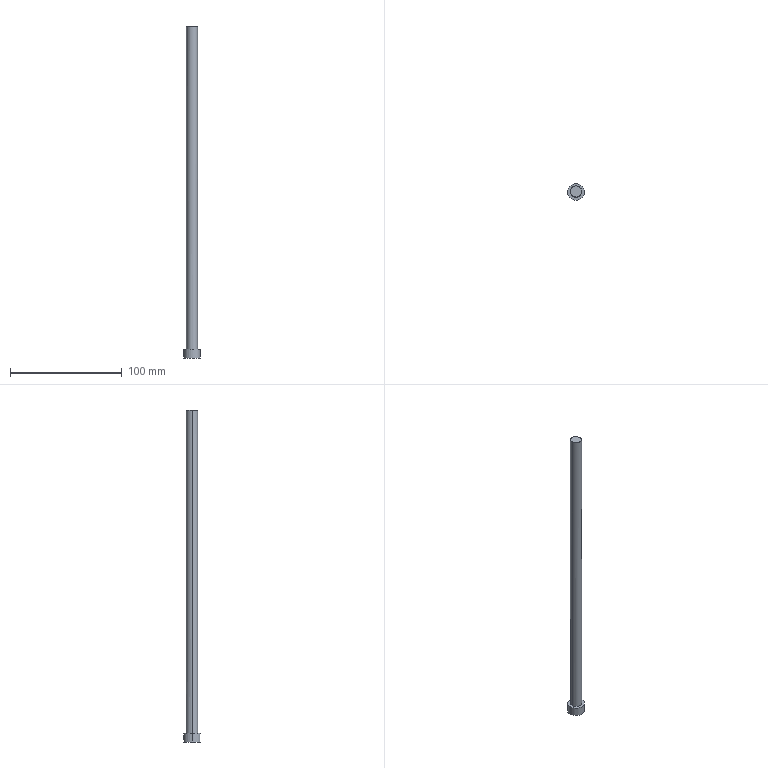Part | Creo | 1 solid | 10 faces | box 15 x 15 x 296.928 mm | volume 24037 mm3 | cylinder 6 | plane 4 | commonest cylinder face diameters 3 x2 10 x2 15 x2
STEP:
#1=CARTESIAN_POINT('',(-35.,201.,-252.5));
#2=VERTEX_POINT('',#1);
#3=CARTESIAN_POINT('',(-25.,201.,-252.5));
#4=VERTEX_POINT('',#3);
#5=CARTESIAN_POINT('',(-30.,201.,-252.5));
#6=DIRECTION('',(0.,0.,-1.));
#7=DIRECTION('',(-1.,0.,0.));
#8=AXIS2_PLACEMENT_3D('',#5,#6,#7);
#9=CIRCLE('',#8,5.);
#10=EDGE_CURVE('',#2,#4,#9,.T.);
#11=ORIENTED_EDGE('',*,*,#10,.T.);
#12=CARTESIAN_POINT('',(-25.,201.,36.046));
#13=VERTEX_POINT('',#12);
#14=CARTESIAN_POINT('',(-25.,201.,36.046));
#15=DIRECTION('',(0.,0.,-1.));
#16=VECTOR('',#15,288.546);
#17=LINE('',#14,#16);
#18=EDGE_CURVE('',#13,#4,#17,.T.);
#19=ORIENTED_EDGE('',*,*,#18,.F.);
#20=CARTESIAN_POINT('',(-35.,201.,36.428));
#21=VERTEX_POINT('',#20);
#22=CARTESIAN_POINT('',(-25.,201.,36.046));
#23=CARTESIAN_POINT('',(-25.,201.589,36.046));
#24=CARTESIAN_POINT('',(-25.215,202.862,36.054));
#25=CARTESIAN_POINT('',(-26.355,204.641,36.098));
#26=CARTESIAN_POINT('',(-28.15,205.786,36.166));
#27=CARTESIAN_POINT('',(-30.,206.107,36.237));
#28=CARTESIAN_POINT('',(-31.85,205.786,36.308));
#29=CARTESIAN_POINT('',(-33.645,204.641,36.376));
#30=CARTESIAN_POINT('',(-34.785,202.862,36.42));
#31=CARTESIAN_POINT('',(-35.,201.589,36.428));
#32=CARTESIAN_POINT('',(-35.,201.,36.428));
#33=B_SPLINE_CURVE_WITH_KNOTS('',3,(#22,#23,#24,#25,#26,#27,#28,#29,#30,#31,#32),.UNSPECIFIED.,.F.,.F.,(4,1,1,1,1,1,1,1,4),(0.,0.125,0.25,0.375,0.5,0.625,0.75,0.875,1.),.UNSPECIFIED.);
#34=EDGE_CURVE('',#13,#21,#33,.T.);
#35=ORIENTED_EDGE('',*,*,#34,.T.);
#36=CARTESIAN_POINT('',(-35.,201.,36.428));
#37=DIRECTION('',(0.,0.,-1.));
#38=VECTOR('',#37,288.928);
#39=LINE('',#36,#38);
#40=EDGE_CURVE('',#21,#2,#39,.T.);
#41=ORIENTED_EDGE('',*,*,#40,.T.);
#42=EDGE_LOOP('',(#11,#19,#35,#41));
#43=FACE_OUTER_BOUND('',#42,.F.);
#44=CARTESIAN_POINT('',(-30.,201.,135.));
#45=DIRECTION('',(0.,0.,-1.));
#46=DIRECTION('',(-1.,0.,0.));
#47=AXIS2_PLACEMENT_3D('',#44,#45,#46);
#48=CYLINDRICAL_SURFACE('',#47,5.);
#49=ADVANCED_FACE('',(#43),#48,.T.);
#50=CARTESIAN_POINT('',(-37.5,201.,-252.5));
#51=VERTEX_POINT('',#50);
#52=CARTESIAN_POINT('',(-22.5,201.,-252.5));
#53=VERTEX_POINT('',#52);
#54=CARTESIAN_POINT('',(-30.,201.,-252.5));
#55=DIRECTION('',(0.,0.,1.));
#56=DIRECTION('',(-1.,0.,0.));
#57=AXIS2_PLACEMENT_3D('',#54,#55,#56);
#58=CIRCLE('',#57,7.5);
#59=EDGE_CURVE('',#51,#53,#58,.T.);
#60=ORIENTED_EDGE('',*,*,#59,.F.);
#61=CARTESIAN_POINT('',(-30.,201.,-252.5));
#62=DIRECTION('',(0.,0.,1.));
#63=DIRECTION('',(1.,0.,0.));
#64=AXIS2_PLACEMENT_3D('',#61,#62,#63);
#65=CIRCLE('',#64,7.5);
#66=EDGE_CURVE('',#53,#51,#65,.T.);
#67=ORIENTED_EDGE('',*,*,#66,.F.);
#68=EDGE_LOOP('',(#60,#67));
#69=FACE_OUTER_BOUND('',#68,.F.);
#70=ORIENTED_EDGE('',*,*,#10,.F.);
#71=CARTESIAN_POINT('',(-30.,201.,-252.5));
#72=DIRECTION('',(0.,0.,-1.));
#73=DIRECTION('',(1.,0.,0.));
#74=AXIS2_PLACEMENT_3D('',#71,#72,#73);
#75=CIRCLE('',#74,5.);
#76=EDGE_CURVE('',#4,#2,#75,.T.);
#77=ORIENTED_EDGE('',*,*,#76,.F.);
#78=EDGE_LOOP('',(#70,#77));
#79=FACE_BOUND('',#78,.F.);
#80=CARTESIAN_POINT('',(-30.,201.,-252.5));
#81=DIRECTION('',(0.,0.,1.));
#82=DIRECTION('',(-1.,0.,0.));
#83=AXIS2_PLACEMENT_3D('',#80,#81,#82);
#84=PLANE('',#83);
#85=ADVANCED_FACE('',(#69,#79),#84,.T.);
#86=ORIENTED_EDGE('',*,*,#76,.T.);
#87=ORIENTED_EDGE('',*,*,#40,.F.);
#88=CARTESIAN_POINT('',(-35.,201.,36.428));
#89=CARTESIAN_POINT('',(-35.,200.411,36.428));
#90=CARTESIAN_POINT('',(-34.785,199.138,36.42));
#91=CARTESIAN_POINT('',(-33.645,197.359,36.376));
#92=CARTESIAN_POINT('',(-31.85,196.214,36.308));
#93=CARTESIAN_POINT('',(-30.,195.893,36.237));
#94=CARTESIAN_POINT('',(-28.15,196.214,36.166));
#95=CARTESIAN_POINT('',(-26.355,197.359,36.098));
#96=CARTESIAN_POINT('',(-25.215,199.138,36.054));
#97=CARTESIAN_POINT('',(-25.,200.411,36.046));
#98=CARTESIAN_POINT('',(-25.,201.,36.046));
#99=B_SPLINE_CURVE_WITH_KNOTS('',3,(#88,#89,#90,#91,#92,#93,#94,#95,#96,#97,#98),.UNSPECIFIED.,.F.,.F.,(4,1,1,1,1,1,1,1,4),(0.,0.125,0.25,0.375,0.5,0.625,0.75,0.875,1.),.UNSPECIFIED.);
#100=EDGE_CURVE('',#21,#13,#99,.T.);
#101=ORIENTED_EDGE('',*,*,#100,.T.);
#102=ORIENTED_EDGE('',*,*,#18,.T.);
#103=EDGE_LOOP('',(#86,#87,#101,#102));
#104=FACE_OUTER_BOUND('',#103,.F.);
#105=CARTESIAN_POINT('',(-30.,201.,135.));
#106=DIRECTION('',(0.,0.,-1.));
#107=DIRECTION('',(-1.,0.,0.));
#108=AXIS2_PLACEMENT_3D('',#105,#106,#107);
#109=CYLINDRICAL_SURFACE('',#108,5.);
#110=ADVANCED_FACE('',(#104),#109,.T.);
#111=ORIENTED_EDGE('',*,*,#34,.F.);
#112=ORIENTED_EDGE('',*,*,#100,.F.);
#113=EDGE_LOOP('',(#111,#112));
#114=FACE_OUTER_BOUND('',#113,.F.);
#115=CARTESIAN_POINT('',(0.9569,33.474,35.055));
#116=DIRECTION('',(0.03814,0.,0.9993));
#117=DIRECTION('',(0.9993,0.,-0.03814));
#118=AXIS2_PLACEMENT_3D('',#115,#116,#117);
#119=PLANE('',#118);
#120=ADVANCED_FACE('',(#114),#119,.T.);
#121=ORIENTED_EDGE('',*,*,#59,.T.);
#122=CARTESIAN_POINT('',(-22.5,201.,-260.5));
#123=VERTEX_POINT('',#122);
#124=CARTESIAN_POINT('',(-22.5,201.,-260.5));
#125=DIRECTION('',(0.,0.,1.));
#126=VECTOR('',#125,8.);
#127=LINE('',#124,#126);
#128=EDGE_CURVE('',#123,#53,#127,.T.);
#129=ORIENTED_EDGE('',*,*,#128,.F.);
#130=CARTESIAN_POINT('',(-37.5,201.,-260.5));
#131=VERTEX_POINT('',#130);
#132=CARTESIAN_POINT('',(-30.,201.,-260.5));
#133=DIRECTION('',(0.,0.,-1.));
#134=DIRECTION('',(1.,0.,0.));
#135=AXIS2_PLACEMENT_3D('',#132,#133,#134);
#136=CIRCLE('',#135,7.5);
#137=EDGE_CURVE('',#123,#131,#136,.T.);
#138=ORIENTED_EDGE('',*,*,#137,.T.);
#139=CARTESIAN_POINT('',(-37.5,201.,-260.5));
#140=DIRECTION('',(0.,0.,1.));
#141=VECTOR('',#140,8.);
#142=LINE('',#139,#141);
#143=EDGE_CURVE('',#131,#51,#142,.T.);
#144=ORIENTED_EDGE('',*,*,#143,.T.);
#145=EDGE_LOOP('',(#121,#129,#138,#144));
#146=FACE_OUTER_BOUND('',#145,.F.);
#147=CARTESIAN_POINT('',(-30.,201.,-260.5));
#148=DIRECTION('',(0.,0.,1.));
#149=DIRECTION('',(-1.,0.,0.));
#150=AXIS2_PLACEMENT_3D('',#147,#148,#149);
#151=CYLINDRICAL_SURFACE('',#150,7.5);
#152=ADVANCED_FACE('',(#146),#151,.T.);
#153=ORIENTED_EDGE('',*,*,#66,.T.);
#154=ORIENTED_EDGE('',*,*,#143,.F.);
#155=CARTESIAN_POINT('',(-30.,201.,-260.5));
#156=DIRECTION('',(0.,0.,-1.));
#157=DIRECTION('',(-1.,0.,0.));
#158=AXIS2_PLACEMENT_3D('',#155,#156,#157);
#159=CIRCLE('',#158,7.5);
#160=EDGE_CURVE('',#131,#123,#159,.T.);
#161=ORIENTED_EDGE('',*,*,#160,.T.);
#162=ORIENTED_EDGE('',*,*,#128,.T.);
#163=EDGE_LOOP('',(#153,#154,#161,#162));
#164=FACE_OUTER_BOUND('',#163,.F.);
#165=CARTESIAN_POINT('',(-30.,208.5,-258.));
#166=VERTEX_POINT('',#165);
#167=CARTESIAN_POINT('',(-30.,208.5,-255.));
#168=VERTEX_POINT('',#167);
#169=CARTESIAN_POINT('',(-30.,208.5,-258.));
#170=CARTESIAN_POINT('',(-29.795,208.5,-258.));
#171=CARTESIAN_POINT('',(-29.417,208.484,-257.922));
#172=CARTESIAN_POINT('',(-28.91,208.425,-257.589));
#173=CARTESIAN_POINT('',(-28.576,208.365,-257.085));
#174=CARTESIAN_POINT('',(-28.461,208.34,-256.497));
#175=CARTESIAN_POINT('',(-28.578,208.365,-255.912));
#176=CARTESIAN_POINT('',(-28.909,208.425,-255.413));
#177=CARTESIAN_POINT('',(-29.415,208.484,-255.078));
#178=CARTESIAN_POINT('',(-29.794,208.5,-255.));
#179=CARTESIAN_POINT('',(-30.,208.5,-255.));
#180=B_SPLINE_CURVE_WITH_KNOTS('',3,(#169,#170,#171,#172,#173,#174,#175,#176,#177,#178,#179),.UNSPECIFIED.,.F.,.F.,(4,1,1,1,1,1,1,1,4),(0.,0.125,0.25,0.375,0.5,0.625,0.75,0.875,1.),.UNSPECIFIED.);
#181=EDGE_CURVE('',#166,#168,#180,.T.);
#182=ORIENTED_EDGE('',*,*,#181,.F.);
#183=CARTESIAN_POINT('',(-30.,208.5,-255.));
#184=CARTESIAN_POINT('',(-30.206,208.5,-255.));
#185=CARTESIAN_POINT('',(-30.585,208.484,-255.078));
#186=CARTESIAN_POINT('',(-31.093,208.424,-255.414));
#187=CARTESIAN_POINT('',(-31.424,208.364,-255.917));
#188=CARTESIAN_POINT('',(-31.539,208.34,-256.506));
#189=CARTESIAN_POINT('',(-31.421,208.365,-257.089));
#190=CARTESIAN_POINT('',(-31.092,208.424,-257.586));
#191=CARTESIAN_POINT('',(-30.586,208.484,-257.922));
#192=CARTESIAN_POINT('',(-30.206,208.5,-258.));
#193=CARTESIAN_POINT('',(-30.,208.5,-258.));
#194=B_SPLINE_CURVE_WITH_KNOTS('',3,(#183,#184,#185,#186,#187,#188,#189,#190,#191,#192,#193),.UNSPECIFIED.,.F.,.F.,(4,1,1,1,1,1,1,1,4),(0.,0.125,0.25,0.375,0.5,0.625,0.75,0.875,1.),.UNSPECIFIED.);
#195=EDGE_CURVE('',#168,#166,#194,.T.);
#196=ORIENTED_EDGE('',*,*,#195,.F.);
#197=EDGE_LOOP('',(#182,#196));
#198=FACE_BOUND('',#197,.F.);
#199=CARTESIAN_POINT('',(-30.,201.,-260.5));
#200=DIRECTION('',(0.,0.,1.));
#201=DIRECTION('',(-1.,0.,0.));
#202=AXIS2_PLACEMENT_3D('',#199,#200,#201);
#203=CYLINDRICAL_SURFACE('',#202,7.5);
#204=ADVANCED_FACE('',(#164,#198),#203,.T.);
#205=ORIENTED_EDGE('',*,*,#181,.T.);
#206=CARTESIAN_POINT('',(-30.,201.,-255.));
#207=VERTEX_POINT('',#206);
#208=CARTESIAN_POINT('',(-30.,201.,-255.));
#209=DIRECTION('',(-0.000000004,1.,-0.000006083));
#210=VECTOR('',#209,7.5);
#211=LINE('',#208,#210);
#212=EDGE_CURVE('',#207,#168,#211,.T.);
#213=ORIENTED_EDGE('',*,*,#212,.F.);
#214=CARTESIAN_POINT('',(-30.,201.,-258.));
#215=VERTEX_POINT('',#214);
#216=CARTESIAN_POINT('',(-30.,201.,-256.5));
#217=DIRECTION('',(0.,1.,0.));
#218=DIRECTION('',(0.,0.,1.));
#219=AXIS2_PLACEMENT_3D('',#216,#217,#218);
#220=CIRCLE('',#219,1.5);
#221=EDGE_CURVE('',#207,#215,#220,.T.);
#222=ORIENTED_EDGE('',*,*,#221,.T.);
#223=CARTESIAN_POINT('',(-30.,201.,-258.));
#224=DIRECTION('',(0.,1.,0.));
#225=VECTOR('',#224,7.5);
#226=LINE('',#223,#225);
#227=EDGE_CURVE('',#215,#166,#226,.T.);
#228=ORIENTED_EDGE('',*,*,#227,.T.);
#229=EDGE_LOOP('',(#205,#213,#222,#228));
#230=FACE_OUTER_BOUND('',#229,.F.);
#231=CARTESIAN_POINT('',(-30.,201.,-256.5));
#232=DIRECTION('',(0.,1.,0.));
#233=DIRECTION('',(0.,0.,-1.));
#234=AXIS2_PLACEMENT_3D('',#231,#232,#233);
#235=CYLINDRICAL_SURFACE('',#234,1.5);
#236=ADVANCED_FACE('',(#230),#235,.F.);
#237=ORIENTED_EDGE('',*,*,#195,.T.);
#238=ORIENTED_EDGE('',*,*,#227,.F.);
#239=CARTESIAN_POINT('',(-30.,201.,-256.5));
#240=DIRECTION('',(0.,1.,0.));
#241=DIRECTION('',(0.,0.,-1.));
#242=AXIS2_PLACEMENT_3D('',#239,#240,#241);
#243=CIRCLE('',#242,1.5);
#244=EDGE_CURVE('',#215,#207,#243,.T.);
#245=ORIENTED_EDGE('',*,*,#244,.T.);
#246=ORIENTED_EDGE('',*,*,#212,.T.);
#247=EDGE_LOOP('',(#237,#238,#245,#246));
#248=FACE_OUTER_BOUND('',#247,.F.);
#249=CARTESIAN_POINT('',(-30.,201.,-256.5));
#250=DIRECTION('',(0.,1.,0.));
#251=DIRECTION('',(0.,0.,-1.));
#252=AXIS2_PLACEMENT_3D('',#249,#250,#251);
#253=CYLINDRICAL_SURFACE('',#252,1.5);
#254=ADVANCED_FACE('',(#248),#253,.F.);
#255=ORIENTED_EDGE('',*,*,#244,.F.);
#256=ORIENTED_EDGE('',*,*,#221,.F.);
#257=EDGE_LOOP('',(#255,#256));
#258=FACE_OUTER_BOUND('',#257,.F.);
#259=CARTESIAN_POINT('',(-30.,201.,-256.5));
#260=DIRECTION('',(0.,-1.,0.));
#261=DIRECTION('',(0.,0.,1.));
#262=AXIS2_PLACEMENT_3D('',#259,#260,#261);
#263=PLANE('',#262);
#264=ADVANCED_FACE('',(#258),#263,.F.);
#265=ORIENTED_EDGE('',*,*,#137,.F.);
#266=ORIENTED_EDGE('',*,*,#160,.F.);
#267=EDGE_LOOP('',(#265,#266));
#268=FACE_OUTER_BOUND('',#267,.F.);
#269=CARTESIAN_POINT('',(7.286,343.015,-260.5));
#270=DIRECTION('',(0.,0.,-1.));
#271=DIRECTION('',(1.,0.,0.));
#272=AXIS2_PLACEMENT_3D('',#269,#270,#271);
#273=PLANE('',#272);
#274=ADVANCED_FACE('',(#268),#273,.T.);
#275=CLOSED_SHELL('',(#49,#85,#110,#120,#152,#204,#236,#254,#264,#274));
#276=MANIFOLD_SOLID_BREP('',#275);
#277=(LENGTH_UNIT()NAMED_UNIT(*)SI_UNIT(.MILLI.,.METRE.));
#278=UNCERTAINTY_MEASURE_WITH_UNIT(LENGTH_MEASURE(0.02977),#277,'','');
#279=(NAMED_UNIT(*)PLANE_ANGLE_UNIT()SI_UNIT($,.RADIAN.));
#280=PLANE_ANGLE_MEASURE_WITH_UNIT(PLANE_ANGLE_MEASURE(0.01745),#279);
#281=(CONVERSION_BASED_UNIT('DEGREE',#280)NAMED_UNIT(*)PLANE_ANGLE_UNIT());
#282=(NAMED_UNIT(*)SI_UNIT($,.STERADIAN.)SOLID_ANGLE_UNIT());
#283=(GEOMETRIC_REPRESENTATION_CONTEXT(3)GLOBAL_UNCERTAINTY_ASSIGNED_CONTEXT((#278))GLOBAL_UNIT_ASSIGNED_CONTEXT((#277,#281,#282))REPRESENTATION_CONTEXT('',''));
#284=ADVANCED_BREP_SHAPE_REPRESENTATION('',(#276),#283);